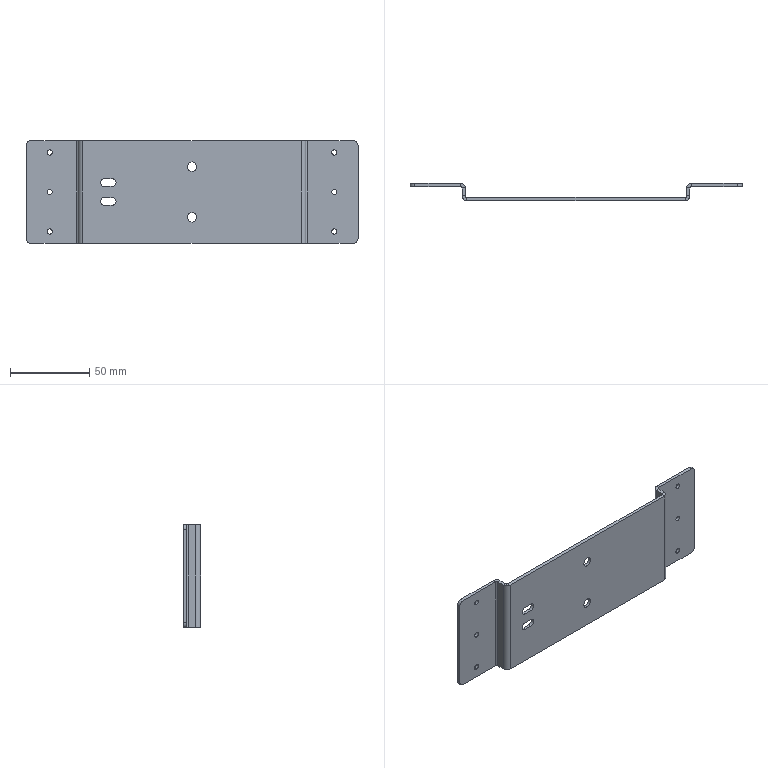Part | SolidWorks | features BaseBody 1 | 1 solid | 66 faces | box 210 x 11 x 65 mm | volume 28784 mm3 | plane 34 | cylinder 32 | commonest cylinder face diameters 3.3 x12 6 x12 2 x4 5 x4